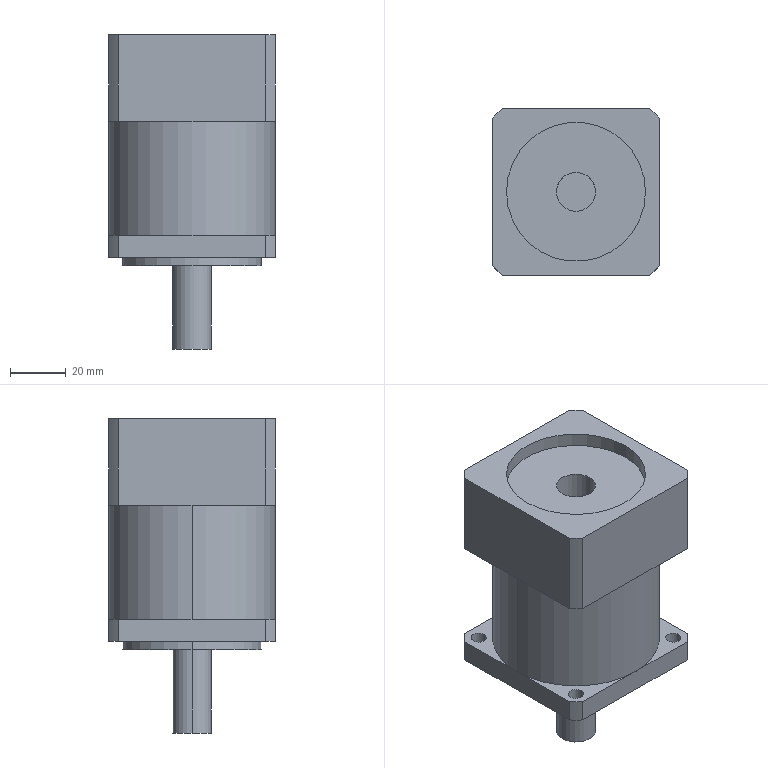Part | SolidWorks | features ICE 7, Extrusion 1, RefAxis 1, RevCut 1 | 1 solid | 48 faces | box 60 x 60 x 113 mm | volume 251469 mm3 | cylinder 26 | plane 22 | commonest cylinder face diameters 5.5 x8 80 x8 14 x4 50 x4 60 x2
STEP:
#1=CARTESIAN_POINT('',(-7.,0.,83.));
#2=VERTEX_POINT('',#1);
#3=CARTESIAN_POINT('',(7.,0.,83.));
#4=VERTEX_POINT('',#3);
#5=CARTESIAN_POINT('',(0.,0.,83.));
#6=DIRECTION('',(0.,0.,1.));
#7=DIRECTION('',(1.,0.,0.));
#8=AXIS2_PLACEMENT_3D('',#5,#6,#7);
#9=CIRCLE('',#8,7.);
#10=EDGE_CURVE('',#2,#4,#9,.T.);
#11=ORIENTED_EDGE('',*,*,#10,.F.);
#12=CARTESIAN_POINT('',(-7.,0.,108.));
#13=VERTEX_POINT('',#12);
#14=CARTESIAN_POINT('',(-7.,0.,83.));
#15=DIRECTION('',(0.,0.,1.));
#16=VECTOR('',#15,1000.);
#17=LINE('',#14,#16);
#18=EDGE_CURVE('',#2,#13,#17,.T.);
#19=ORIENTED_EDGE('',*,*,#18,.T.);
#20=CARTESIAN_POINT('',(7.,0.,108.));
#21=VERTEX_POINT('',#20);
#22=CARTESIAN_POINT('',(0.,0.,108.));
#23=DIRECTION('',(0.,0.,1.));
#24=DIRECTION('',(1.,0.,0.));
#25=AXIS2_PLACEMENT_3D('',#22,#23,#24);
#26=CIRCLE('',#25,7.);
#27=EDGE_CURVE('',#13,#21,#26,.T.);
#28=ORIENTED_EDGE('',*,*,#27,.T.);
#29=CARTESIAN_POINT('',(7.,0.,83.));
#30=DIRECTION('',(0.,0.,1.));
#31=VECTOR('',#30,1000.);
#32=LINE('',#29,#31);
#33=EDGE_CURVE('',#4,#21,#32,.T.);
#34=ORIENTED_EDGE('',*,*,#33,.F.);
#35=EDGE_LOOP('',(#11,#19,#28,#34));
#36=FACE_OUTER_BOUND('',#35,.T.);
#37=CARTESIAN_POINT('',(0.,0.,83.));
#38=DIRECTION('',(0.,0.,1.));
#39=DIRECTION('',(1.,0.,0.));
#40=AXIS2_PLACEMENT_3D('',#37,#38,#39);
#41=CYLINDRICAL_SURFACE('',#40,7.);
#42=ADVANCED_FACE('',(#36),#41,.F.);
#43=CARTESIAN_POINT('',(-25.,0.,108.));
#44=VERTEX_POINT('',#43);
#45=CARTESIAN_POINT('',(25.,0.,108.));
#46=VERTEX_POINT('',#45);
#47=CARTESIAN_POINT('',(0.,0.,108.));
#48=DIRECTION('',(0.,0.,1.));
#49=DIRECTION('',(1.,0.,0.));
#50=AXIS2_PLACEMENT_3D('',#47,#48,#49);
#51=CIRCLE('',#50,25.);
#52=EDGE_CURVE('',#44,#46,#51,.T.);
#53=ORIENTED_EDGE('',*,*,#52,.F.);
#54=CARTESIAN_POINT('',(-25.,0.,113.));
#55=VERTEX_POINT('',#54);
#56=CARTESIAN_POINT('',(-25.,0.,108.));
#57=DIRECTION('',(0.,0.,1.));
#58=VECTOR('',#57,1000.);
#59=LINE('',#56,#58);
#60=EDGE_CURVE('',#44,#55,#59,.T.);
#61=ORIENTED_EDGE('',*,*,#60,.T.);
#62=CARTESIAN_POINT('',(25.,0.,113.));
#63=VERTEX_POINT('',#62);
#64=CARTESIAN_POINT('',(0.,0.,113.));
#65=DIRECTION('',(0.,0.,1.));
#66=DIRECTION('',(1.,0.,0.));
#67=AXIS2_PLACEMENT_3D('',#64,#65,#66);
#68=CIRCLE('',#67,25.);
#69=EDGE_CURVE('',#55,#63,#68,.T.);
#70=ORIENTED_EDGE('',*,*,#69,.T.);
#71=CARTESIAN_POINT('',(25.,0.,108.));
#72=DIRECTION('',(0.,0.,1.));
#73=VECTOR('',#72,1000.);
#74=LINE('',#71,#73);
#75=EDGE_CURVE('',#46,#63,#74,.T.);
#76=ORIENTED_EDGE('',*,*,#75,.F.);
#77=EDGE_LOOP('',(#53,#61,#70,#76));
#78=FACE_OUTER_BOUND('',#77,.T.);
#79=CARTESIAN_POINT('',(0.,0.,108.));
#80=DIRECTION('',(0.,0.,1.));
#81=DIRECTION('',(1.,0.,0.));
#82=AXIS2_PLACEMENT_3D('',#79,#80,#81);
#83=CYLINDRICAL_SURFACE('',#82,25.);
#84=ADVANCED_FACE('',(#78),#83,.F.);
#85=CARTESIAN_POINT('',(-21.999,24.749,41.));
#86=VERTEX_POINT('',#85);
#87=CARTESIAN_POINT('',(-27.499,24.749,41.));
#88=VERTEX_POINT('',#87);
#89=CARTESIAN_POINT('',(-24.749,24.749,41.));
#90=DIRECTION('',(0.,0.,-1.));
#91=DIRECTION('',(1.,0.,0.));
#92=AXIS2_PLACEMENT_3D('',#89,#90,#91);
#93=CIRCLE('',#92,2.75);
#94=EDGE_CURVE('',#86,#88,#93,.T.);
#95=ORIENTED_EDGE('',*,*,#94,.F.);
#96=CARTESIAN_POINT('',(-21.999,24.749,33.));
#97=VERTEX_POINT('',#96);
#98=CARTESIAN_POINT('',(-21.999,24.749,113.001));
#99=DIRECTION('',(0.,0.,-1.));
#100=VECTOR('',#99,1000.);
#101=LINE('',#98,#100);
#102=EDGE_CURVE('',#86,#97,#101,.T.);
#103=ORIENTED_EDGE('',*,*,#102,.T.);
#104=CARTESIAN_POINT('',(-27.499,24.749,33.));
#105=VERTEX_POINT('',#104);
#106=CARTESIAN_POINT('',(-24.749,24.749,33.));
#107=DIRECTION('',(0.,0.,-1.));
#108=DIRECTION('',(1.,0.,0.));
#109=AXIS2_PLACEMENT_3D('',#106,#107,#108);
#110=CIRCLE('',#109,2.75);
#111=EDGE_CURVE('',#97,#105,#110,.T.);
#112=ORIENTED_EDGE('',*,*,#111,.T.);
#113=CARTESIAN_POINT('',(-27.499,24.749,113.001));
#114=DIRECTION('',(0.,0.,-1.));
#115=VECTOR('',#114,1000.);
#116=LINE('',#113,#115);
#117=EDGE_CURVE('',#88,#105,#116,.T.);
#118=ORIENTED_EDGE('',*,*,#117,.F.);
#119=EDGE_LOOP('',(#95,#103,#112,#118));
#120=FACE_OUTER_BOUND('',#119,.T.);
#121=CARTESIAN_POINT('',(-24.749,24.749,113.001));
#122=DIRECTION('',(0.,0.,-1.));
#123=DIRECTION('',(-1.,0.,0.));
#124=AXIS2_PLACEMENT_3D('',#121,#122,#123);
#125=CYLINDRICAL_SURFACE('',#124,2.75);
#126=ADVANCED_FACE('',(#120),#125,.F.);
#127=CARTESIAN_POINT('',(27.499,-24.749,41.));
#128=VERTEX_POINT('',#127);
#129=CARTESIAN_POINT('',(21.999,-24.749,41.));
#130=VERTEX_POINT('',#129);
#131=CARTESIAN_POINT('',(24.749,-24.749,41.));
#132=DIRECTION('',(0.,0.,-1.));
#133=DIRECTION('',(1.,0.,0.));
#134=AXIS2_PLACEMENT_3D('',#131,#132,#133);
#135=CIRCLE('',#134,2.75);
#136=EDGE_CURVE('',#128,#130,#135,.T.);
#137=ORIENTED_EDGE('',*,*,#136,.F.);
#138=CARTESIAN_POINT('',(27.499,-24.749,33.));
#139=VERTEX_POINT('',#138);
#140=CARTESIAN_POINT('',(27.499,-24.749,113.001));
#141=DIRECTION('',(0.,0.,-1.));
#142=VECTOR('',#141,1000.);
#143=LINE('',#140,#142);
#144=EDGE_CURVE('',#128,#139,#143,.T.);
#145=ORIENTED_EDGE('',*,*,#144,.T.);
#146=CARTESIAN_POINT('',(21.999,-24.749,33.));
#147=VERTEX_POINT('',#146);
#148=CARTESIAN_POINT('',(24.749,-24.749,33.));
#149=DIRECTION('',(0.,0.,-1.));
#150=DIRECTION('',(1.,0.,0.));
#151=AXIS2_PLACEMENT_3D('',#148,#149,#150);
#152=CIRCLE('',#151,2.75);
#153=EDGE_CURVE('',#139,#147,#152,.T.);
#154=ORIENTED_EDGE('',*,*,#153,.T.);
#155=CARTESIAN_POINT('',(21.999,-24.749,113.001));
#156=DIRECTION('',(0.,0.,-1.));
#157=VECTOR('',#156,1000.);
#158=LINE('',#155,#157);
#159=EDGE_CURVE('',#130,#147,#158,.T.);
#160=ORIENTED_EDGE('',*,*,#159,.F.);
#161=EDGE_LOOP('',(#137,#145,#154,#160));
#162=FACE_OUTER_BOUND('',#161,.T.);
#163=CARTESIAN_POINT('',(24.749,-24.749,113.001));
#164=DIRECTION('',(0.,0.,-1.));
#165=DIRECTION('',(-1.,0.,0.));
#166=AXIS2_PLACEMENT_3D('',#163,#164,#165);
#167=CYLINDRICAL_SURFACE('',#166,2.75);
#168=ADVANCED_FACE('',(#162),#167,.F.);
#169=CARTESIAN_POINT('',(-21.999,-24.749,41.));
#170=VERTEX_POINT('',#169);
#171=CARTESIAN_POINT('',(-27.499,-24.749,41.));
#172=VERTEX_POINT('',#171);
#173=CARTESIAN_POINT('',(-24.749,-24.749,41.));
#174=DIRECTION('',(0.,0.,-1.));
#175=DIRECTION('',(1.,0.,0.));
#176=AXIS2_PLACEMENT_3D('',#173,#174,#175);
#177=CIRCLE('',#176,2.75);
#178=EDGE_CURVE('',#170,#172,#177,.T.);
#179=ORIENTED_EDGE('',*,*,#178,.F.);
#180=CARTESIAN_POINT('',(-21.999,-24.749,33.));
#181=VERTEX_POINT('',#180);
#182=CARTESIAN_POINT('',(-21.999,-24.749,113.001));
#183=DIRECTION('',(0.,0.,-1.));
#184=VECTOR('',#183,1000.);
#185=LINE('',#182,#184);
#186=EDGE_CURVE('',#170,#181,#185,.T.);
#187=ORIENTED_EDGE('',*,*,#186,.T.);
#188=CARTESIAN_POINT('',(-27.499,-24.749,33.));
#189=VERTEX_POINT('',#188);
#190=CARTESIAN_POINT('',(-24.749,-24.749,33.));
#191=DIRECTION('',(0.,0.,-1.));
#192=DIRECTION('',(-1.,0.,0.));
#193=AXIS2_PLACEMENT_3D('',#190,#191,#192);
#194=CIRCLE('',#193,2.75);
#195=EDGE_CURVE('',#181,#189,#194,.T.);
#196=ORIENTED_EDGE('',*,*,#195,.T.);
#197=CARTESIAN_POINT('',(-27.499,-24.749,113.001));
#198=DIRECTION('',(0.,0.,-1.));
#199=VECTOR('',#198,1000.);
#200=LINE('',#197,#199);
#201=EDGE_CURVE('',#172,#189,#200,.T.);
#202=ORIENTED_EDGE('',*,*,#201,.F.);
#203=EDGE_LOOP('',(#179,#187,#196,#202));
#204=FACE_OUTER_BOUND('',#203,.T.);
#205=CARTESIAN_POINT('',(-24.749,-24.749,113.001));
#206=DIRECTION('',(0.,0.,-1.));
#207=DIRECTION('',(-1.,0.,0.));
#208=AXIS2_PLACEMENT_3D('',#205,#206,#207);
#209=CYLINDRICAL_SURFACE('',#208,2.75);
#210=ADVANCED_FACE('',(#204),#209,.F.);
#211=CARTESIAN_POINT('',(27.499,24.749,41.));
#212=VERTEX_POINT('',#211);
#213=CARTESIAN_POINT('',(21.999,24.749,41.));
#214=VERTEX_POINT('',#213);
#215=CARTESIAN_POINT('',(24.749,24.749,41.));
#216=DIRECTION('',(0.,0.,-1.));
#217=DIRECTION('',(1.,0.,0.));
#218=AXIS2_PLACEMENT_3D('',#215,#216,#217);
#219=CIRCLE('',#218,2.75);
#220=EDGE_CURVE('',#212,#214,#219,.T.);
#221=ORIENTED_EDGE('',*,*,#220,.F.);
#222=CARTESIAN_POINT('',(27.499,24.749,33.));
#223=VERTEX_POINT('',#222);
#224=CARTESIAN_POINT('',(27.499,24.749,113.001));
#225=DIRECTION('',(0.,0.,-1.));
#226=VECTOR('',#225,1000.);
#227=LINE('',#224,#226);
#228=EDGE_CURVE('',#212,#223,#227,.T.);
#229=ORIENTED_EDGE('',*,*,#228,.T.);
#230=CARTESIAN_POINT('',(21.999,24.749,33.));
#231=VERTEX_POINT('',#230);
#232=CARTESIAN_POINT('',(24.749,24.749,33.));
#233=DIRECTION('',(0.,0.,-1.));
#234=DIRECTION('',(-1.,0.,0.));
#235=AXIS2_PLACEMENT_3D('',#232,#233,#234);
#236=CIRCLE('',#235,2.75);
#237=EDGE_CURVE('',#223,#231,#236,.T.);
#238=ORIENTED_EDGE('',*,*,#237,.T.);
#239=CARTESIAN_POINT('',(21.999,24.749,113.001));
#240=DIRECTION('',(0.,0.,-1.));
#241=VECTOR('',#240,1000.);
#242=LINE('',#239,#241);
#243=EDGE_CURVE('',#214,#231,#242,.T.);
#244=ORIENTED_EDGE('',*,*,#243,.F.);
#245=EDGE_LOOP('',(#221,#229,#238,#244));
#246=FACE_OUTER_BOUND('',#245,.T.);
#247=CARTESIAN_POINT('',(24.749,24.749,113.001));
#248=DIRECTION('',(0.,0.,-1.));
#249=DIRECTION('',(-1.,0.,0.));
#250=AXIS2_PLACEMENT_3D('',#247,#248,#249);
#251=CYLINDRICAL_SURFACE('',#250,2.75);
#252=ADVANCED_FACE('',(#246),#251,.F.);
#253=CARTESIAN_POINT('',(30.,0.,82.));
#254=VERTEX_POINT('',#253);
#255=CARTESIAN_POINT('',(0.,30.,82.));
#256=VERTEX_POINT('',#255);
#257=CARTESIAN_POINT('',(0.,0.,82.));
#258=DIRECTION('',(0.,0.,1.));
#259=DIRECTION('',(1.,0.,0.));
#260=AXIS2_PLACEMENT_3D('',#257,#258,#259);
#261=CIRCLE('',#260,30.);
#262=EDGE_CURVE('',#254,#256,#261,.T.);
#263=ORIENTED_EDGE('',*,*,#262,.F.);
#264=CARTESIAN_POINT('',(30.,0.,41.));
#265=VERTEX_POINT('',#264);
#266=CARTESIAN_POINT('',(30.,0.,82.));
#267=DIRECTION('',(0.,0.,-1.));
#268=VECTOR('',#267,1000.);
#269=LINE('',#266,#268);
#270=EDGE_CURVE('',#254,#265,#269,.T.);
#271=ORIENTED_EDGE('',*,*,#270,.T.);
#272=CARTESIAN_POINT('',(0.,30.,41.));
#273=VERTEX_POINT('',#272);
#274=CARTESIAN_POINT('',(0.,0.,41.));
#275=DIRECTION('',(0.,0.,1.));
#276=DIRECTION('',(1.,0.,0.));
#277=AXIS2_PLACEMENT_3D('',#274,#275,#276);
#278=CIRCLE('',#277,30.);
#279=EDGE_CURVE('',#265,#273,#278,.T.);
#280=ORIENTED_EDGE('',*,*,#279,.T.);
#281=CARTESIAN_POINT('',(-30.,0.,41.));
#282=VERTEX_POINT('',#281);
#283=CARTESIAN_POINT('',(0.,0.,41.));
#284=DIRECTION('',(0.,0.,1.));
#285=DIRECTION('',(1.,0.,0.));
#286=AXIS2_PLACEMENT_3D('',#283,#284,#285);
#287=CIRCLE('',#286,30.);
#288=EDGE_CURVE('',#273,#282,#287,.T.);
#289=ORIENTED_EDGE('',*,*,#288,.T.);
#290=CARTESIAN_POINT('',(-30.,0.,82.));
#291=VERTEX_POINT('',#290);
#292=CARTESIAN_POINT('',(-30.,0.,82.));
#293=DIRECTION('',(0.,0.,-1.));
#294=VECTOR('',#293,1000.);
#295=LINE('',#292,#294);
#296=EDGE_CURVE('',#291,#282,#295,.T.);
#297=ORIENTED_EDGE('',*,*,#296,.F.);
#298=CARTESIAN_POINT('',(0.,0.,82.));
#299=DIRECTION('',(0.,0.,1.));
#300=DIRECTION('',(1.,0.,0.));
#301=AXIS2_PLACEMENT_3D('',#298,#299,#300);
#302=CIRCLE('',#301,30.);
#303=EDGE_CURVE('',#256,#291,#302,.T.);
#304=ORIENTED_EDGE('',*,*,#303,.F.);
#305=EDGE_LOOP('',(#263,#271,#280,#289,#297,#304));
#306=FACE_OUTER_BOUND('',#305,.T.);
#307=CARTESIAN_POINT('',(0.,0.,82.));
#308=DIRECTION('',(0.,0.,-1.));
#309=DIRECTION('',(-1.,0.,0.));
#310=AXIS2_PLACEMENT_3D('',#307,#308,#309);
#311=CYLINDRICAL_SURFACE('',#310,30.);
#312=ADVANCED_FACE('',(#306),#311,.T.);
#313=CARTESIAN_POINT('',(25.,0.,33.));
#314=VERTEX_POINT('',#313);
#315=CARTESIAN_POINT('',(-25.,0.,33.));
#316=VERTEX_POINT('',#315);
#317=CARTESIAN_POINT('',(0.,0.,33.));
#318=DIRECTION('',(0.,0.,1.));
#319=DIRECTION('',(1.,0.,0.));
#320=AXIS2_PLACEMENT_3D('',#317,#318,#319);
#321=CIRCLE('',#320,25.);
#322=EDGE_CURVE('',#314,#316,#321,.T.);
#323=ORIENTED_EDGE('',*,*,#322,.F.);
#324=CARTESIAN_POINT('',(25.,0.,30.));
#325=VERTEX_POINT('',#324);
#326=CARTESIAN_POINT('',(25.,0.,33.));
#327=DIRECTION('',(0.,0.,-1.));
#328=VECTOR('',#327,1000.);
#329=LINE('',#326,#328);
#330=EDGE_CURVE('',#314,#325,#329,.T.);
#331=ORIENTED_EDGE('',*,*,#330,.T.);
#332=CARTESIAN_POINT('',(-25.,0.,30.));
#333=VERTEX_POINT('',#332);
#334=CARTESIAN_POINT('',(0.,0.,30.));
#335=DIRECTION('',(0.,0.,1.));
#336=DIRECTION('',(1.,0.,0.));
#337=AXIS2_PLACEMENT_3D('',#334,#335,#336);
#338=CIRCLE('',#337,25.);
#339=EDGE_CURVE('',#325,#333,#338,.T.);
#340=ORIENTED_EDGE('',*,*,#339,.T.);
#341=CARTESIAN_POINT('',(-25.,0.,33.));
#342=DIRECTION('',(0.,0.,-1.));
#343=VECTOR('',#342,1000.);
#344=LINE('',#341,#343);
#345=EDGE_CURVE('',#316,#333,#344,.T.);
#346=ORIENTED_EDGE('',*,*,#345,.F.);
#347=EDGE_LOOP('',(#323,#331,#340,#346));
#348=FACE_OUTER_BOUND('',#347,.T.);
#349=CARTESIAN_POINT('',(0.,0.,33.));
#350=DIRECTION('',(0.,0.,-1.));
#351=DIRECTION('',(-1.,0.,0.));
#352=AXIS2_PLACEMENT_3D('',#349,#350,#351);
#353=CYLINDRICAL_SURFACE('',#352,25.);
#354=ADVANCED_FACE('',(#348),#353,.T.);
#355=CARTESIAN_POINT('',(7.,0.,30.));
#356=VERTEX_POINT('',#355);
#357=CARTESIAN_POINT('',(-7.,0.,30.));
#358=VERTEX_POINT('',#357);
#359=CARTESIAN_POINT('',(0.,0.,30.));
#360=DIRECTION('',(0.,0.,1.));
#361=DIRECTION('',(1.,0.,0.));
#362=AXIS2_PLACEMENT_3D('',#359,#360,#361);
#363=CIRCLE('',#362,7.);
#364=EDGE_CURVE('',#356,#358,#363,.T.);
#365=ORIENTED_EDGE('',*,*,#364,.F.);
#366=CARTESIAN_POINT('',(7.,0.,0.));
#367=VERTEX_POINT('',#366);
#368=CARTESIAN_POINT('',(7.,0.,30.));
#369=DIRECTION('',(0.,0.,-1.));
#370=VECTOR('',#369,1000.);
#371=LINE('',#368,#370);
#372=EDGE_CURVE('',#356,#367,#371,.T.);
#373=ORIENTED_EDGE('',*,*,#372,.T.);
#374=CARTESIAN_POINT('',(-7.,0.,0.));
#375=VERTEX_POINT('',#374);
#376=CARTESIAN_POINT('',(0.,0.,0.));
#377=DIRECTION('',(0.,0.,1.));
#378=DIRECTION('',(1.,0.,0.));
#379=AXIS2_PLACEMENT_3D('',#376,#377,#378);
#380=CIRCLE('',#379,7.);
#381=EDGE_CURVE('',#367,#375,#380,.T.);
#382=ORIENTED_EDGE('',*,*,#381,.T.);
#383=CARTESIAN_POINT('',(-7.,0.,30.));
#384=DIRECTION('',(0.,0.,-1.));
#385=VECTOR('',#384,1000.);
#386=LINE('',#383,#385);
#387=EDGE_CURVE('',#358,#375,#386,.T.);
#388=ORIENTED_EDGE('',*,*,#387,.F.);
#389=EDGE_LOOP('',(#365,#373,#382,#388));
#390=FACE_OUTER_BOUND('',#389,.T.);
#391=CARTESIAN_POINT('',(0.,0.,30.));
#392=DIRECTION('',(0.,0.,-1.));
#393=DIRECTION('',(-1.,0.,0.));
#394=AXIS2_PLACEMENT_3D('',#391,#392,#393);
#395=CYLINDRICAL_SURFACE('',#394,7.);
#396=ADVANCED_FACE('',(#390),#395,.T.);
#397=CARTESIAN_POINT('',(24.749,24.749,41.));
#398=DIRECTION('',(0.,0.,-1.));
#399=DIRECTION('',(1.,0.,0.));
#400=AXIS2_PLACEMENT_3D('',#397,#398,#399);
#401=CIRCLE('',#400,2.75);
#402=EDGE_CURVE('',#214,#212,#401,.T.);
#403=ORIENTED_EDGE('',*,*,#402,.T.);
#404=ORIENTED_EDGE('',*,*,#220,.T.);
#405=EDGE_LOOP('',(#403,#404));
#406=FACE_BOUND('',#405,.T.);
#407=CARTESIAN_POINT('',(30.,26.458,41.));
#408=VERTEX_POINT('',#407);
#409=CARTESIAN_POINT('',(30.,30.,41.));
#410=DIRECTION('',(0.,1.,0.));
#411=VECTOR('',#410,1000.);
#412=LINE('',#409,#411);
#413=EDGE_CURVE('',#265,#408,#412,.T.);
#414=ORIENTED_EDGE('',*,*,#413,.T.);
#415=CARTESIAN_POINT('',(26.458,30.,41.));
#416=VERTEX_POINT('',#415);
#417=CARTESIAN_POINT('',(0.,0.,41.));
#418=DIRECTION('',(0.,0.,1.));
#419=DIRECTION('',(1.,0.,0.));
#420=AXIS2_PLACEMENT_3D('',#417,#418,#419);
#421=CIRCLE('',#420,40.);
#422=EDGE_CURVE('',#408,#416,#421,.T.);
#423=ORIENTED_EDGE('',*,*,#422,.T.);
#424=CARTESIAN_POINT('',(-30.,30.,41.));
#425=DIRECTION('',(-1.,0.,0.));
#426=VECTOR('',#425,1000.);
#427=LINE('',#424,#426);
#428=EDGE_CURVE('',#416,#273,#427,.T.);
#429=ORIENTED_EDGE('',*,*,#428,.T.);
#430=ORIENTED_EDGE('',*,*,#279,.F.);
#431=EDGE_LOOP('',(#414,#423,#429,#430));
#432=FACE_OUTER_BOUND('',#431,.T.);
#433=CARTESIAN_POINT('',(0.,0.,41.));
#434=DIRECTION('',(0.,0.,1.));
#435=DIRECTION('',(1.,0.,0.));
#436=AXIS2_PLACEMENT_3D('',#433,#434,#435);
#437=PLANE('',#436);
#438=ADVANCED_FACE('',(#406,#432),#437,.T.);
#439=CARTESIAN_POINT('',(-24.749,24.749,41.));
#440=DIRECTION('',(0.,0.,-1.));
#441=DIRECTION('',(1.,0.,0.));
#442=AXIS2_PLACEMENT_3D('',#439,#440,#441);
#443=CIRCLE('',#442,2.75);
#444=EDGE_CURVE('',#88,#86,#443,.T.);
#445=ORIENTED_EDGE('',*,*,#444,.T.);
#446=ORIENTED_EDGE('',*,*,#94,.T.);
#447=EDGE_LOOP('',(#445,#446));
#448=FACE_BOUND('',#447,.T.);
#449=CARTESIAN_POINT('',(-26.458,30.,41.));
#450=VERTEX_POINT('',#449);
#451=CARTESIAN_POINT('',(-30.,30.,41.));
#452=DIRECTION('',(-1.,0.,0.));
#453=VECTOR('',#452,1000.);
#454=LINE('',#451,#453);
#455=EDGE_CURVE('',#273,#450,#454,.T.);
#456=ORIENTED_EDGE('',*,*,#455,.T.);
#457=CARTESIAN_POINT('',(-30.,26.458,41.));
#458=VERTEX_POINT('',#457);
#459=CARTESIAN_POINT('',(0.,0.,41.));
#460=DIRECTION('',(0.,0.,1.));
#461=DIRECTION('',(1.,0.,0.));
#462=AXIS2_PLACEMENT_3D('',#459,#460,#461);
#463=CIRCLE('',#462,40.);
#464=EDGE_CURVE('',#450,#458,#463,.T.);
#465=ORIENTED_EDGE('',*,*,#464,.T.);
#466=CARTESIAN_POINT('',(-30.,30.,41.));
#467=DIRECTION('',(0.,-1.,0.));
#468=VECTOR('',#467,1000.);
#469=LINE('',#466,#468);
#470=EDGE_CURVE('',#458,#282,#469,.T.);
#471=ORIENTED_EDGE('',*,*,#470,.T.);
#472=ORIENTED_EDGE('',*,*,#288,.F.);
#473=EDGE_LOOP('',(#456,#465,#471,#472));
#474=FACE_OUTER_BOUND('',#473,.T.);
#475=CARTESIAN_POINT('',(0.,0.,41.));
#476=DIRECTION('',(0.,0.,1.));
#477=DIRECTION('',(1.,0.,0.));
#478=AXIS2_PLACEMENT_3D('',#475,#476,#477);
#479=PLANE('',#478);
#480=ADVANCED_FACE('',(#448,#474),#479,.T.);
#481=CARTESIAN_POINT('',(-24.749,-24.749,41.));
#482=DIRECTION('',(0.,0.,-1.));
#483=DIRECTION('',(1.,0.,0.));
#484=AXIS2_PLACEMENT_3D('',#481,#482,#483);
#485=CIRCLE('',#484,2.75);
#486=EDGE_CURVE('',#172,#170,#485,.T.);
#487=ORIENTED_EDGE('',*,*,#486,.T.);
#488=ORIENTED_EDGE('',*,*,#178,.T.);
#489=EDGE_LOOP('',(#487,#488));
#490=FACE_BOUND('',#489,.T.);
#491=CARTESIAN_POINT('',(-30.,-26.458,41.));
#492=VERTEX_POINT('',#491);
#493=CARTESIAN_POINT('',(-30.,30.,41.));
#494=DIRECTION('',(0.,-1.,0.));
#495=VECTOR('',#494,1000.);
#496=LINE('',#493,#495);
#497=EDGE_CURVE('',#282,#492,#496,.T.);
#498=ORIENTED_EDGE('',*,*,#497,.T.);
#499=CARTESIAN_POINT('',(-26.458,-30.,41.));
#500=VERTEX_POINT('',#499);
#501=CARTESIAN_POINT('',(0.,0.,41.));
#502=DIRECTION('',(0.,0.,1.));
#503=DIRECTION('',(1.,0.,0.));
#504=AXIS2_PLACEMENT_3D('',#501,#502,#503);
#505=CIRCLE('',#504,40.);
#506=EDGE_CURVE('',#492,#500,#505,.T.);
#507=ORIENTED_EDGE('',*,*,#506,.T.);
#508=CARTESIAN_POINT('',(0.,-30.,41.));
#509=VERTEX_POINT('',#508);
#510=CARTESIAN_POINT('',(-30.,-30.,41.));
#511=DIRECTION('',(1.,0.,0.));
#512=VECTOR('',#511,1000.);
#513=LINE('',#510,#512);
#514=EDGE_CURVE('',#500,#509,#513,.T.);
#515=ORIENTED_EDGE('',*,*,#514,.T.);
#516=CARTESIAN_POINT('',(0.,0.,41.));
#517=DIRECTION('',(0.,0.,1.));
#518=DIRECTION('',(1.,0.,0.));
#519=AXIS2_PLACEMENT_3D('',#516,#517,#518);
#520=CIRCLE('',#519,30.);
#521=EDGE_CURVE('',#282,#509,#520,.T.);
#522=ORIENTED_EDGE('',*,*,#521,.F.);
#523=EDGE_LOOP('',(#498,#507,#515,#522));
#524=FACE_OUTER_BOUND('',#523,.T.);
#525=CARTESIAN_POINT('',(0.,0.,41.));
#526=DIRECTION('',(0.,0.,1.));
#527=DIRECTION('',(1.,0.,0.));
#528=AXIS2_PLACEMENT_3D('',#525,#526,#527);
#529=PLANE('',#528);
#530=ADVANCED_FACE('',(#490,#524),#529,.T.);
#531=CARTESIAN_POINT('',(30.,-26.458,33.));
#532=VERTEX_POINT('',#531);
#533=CARTESIAN_POINT('',(30.,-26.458,41.));
#534=VERTEX_POINT('',#533);
#535=CARTESIAN_POINT('',(30.,-26.458,82.));
#536=DIRECTION('',(0.,0.,1.));
#537=VECTOR('',#536,1000.);
#538=LINE('',#535,#537);
#539=EDGE_CURVE('',#532,#534,#538,.T.);
#540=ORIENTED_EDGE('',*,*,#539,.F.);
#541=CARTESIAN_POINT('',(30.,26.458,33.));
#542=VERTEX_POINT('',#541);
#543=CARTESIAN_POINT('',(30.,30.,33.));
#544=DIRECTION('',(0.,1.,0.));
#545=VECTOR('',#544,1000.);
#546=LINE('',#543,#545);
#547=EDGE_CURVE('',#532,#542,#546,.T.);
#548=ORIENTED_EDGE('',*,*,#547,.T.);
#549=CARTESIAN_POINT('',(30.,26.458,82.));
#550=DIRECTION('',(0.,0.,-1.));
#551=VECTOR('',#550,1000.);
#552=LINE('',#549,#551);
#553=EDGE_CURVE('',#408,#542,#552,.T.);
#554=ORIENTED_EDGE('',*,*,#553,.F.);
#555=ORIENTED_EDGE('',*,*,#413,.F.);
#556=CARTESIAN_POINT('',(30.,30.,41.));
#557=DIRECTION('',(0.,1.,0.));
#558=VECTOR('',#557,1000.);
#559=LINE('',#556,#558);
#560=EDGE_CURVE('',#534,#265,#559,.T.);
#561=ORIENTED_EDGE('',*,*,#560,.F.);
#562=EDGE_LOOP('',(#540,#548,#554,#555,#561));
#563=FACE_OUTER_BOUND('',#562,.T.);
#564=CARTESIAN_POINT('',(30.,30.,41.));
#565=DIRECTION('',(-1.,0.,0.));
#566=DIRECTION('',(0.,-1.,0.));
#567=AXIS2_PLACEMENT_3D('',#564,#565,#566);
#568=PLANE('',#567);
#569=ADVANCED_FACE('',(#563),#568,.F.);
#570=CARTESIAN_POINT('',(26.458,30.,33.));
#571=VERTEX_POINT('',#570);
#572=CARTESIAN_POINT('',(26.458,30.,82.));
#573=DIRECTION('',(0.,0.,1.));
#574=VECTOR('',#573,1000.);
#575=LINE('',#572,#574);
#576=EDGE_CURVE('',#571,#416,#575,.T.);
#577=ORIENTED_EDGE('',*,*,#576,.F.);
#578=CARTESIAN_POINT('',(-26.458,30.,33.));
#579=VERTEX_POINT('',#578);
#580=CARTESIAN_POINT('',(-30.,30.,33.));
#581=DIRECTION('',(-1.,0.,0.));
#582=VECTOR('',#581,1000.);
#583=LINE('',#580,#582);
#584=EDGE_CURVE('',#571,#579,#583,.T.);
#585=ORIENTED_EDGE('',*,*,#584,.T.);
#586=CARTESIAN_POINT('',(-26.458,30.,82.));
#587=DIRECTION('',(0.,0.,-1.));
#588=VECTOR('',#587,1000.);
#589=LINE('',#586,#588);
#590=EDGE_CURVE('',#450,#579,#589,.T.);
#591=ORIENTED_EDGE('',*,*,#590,.F.);
#592=ORIENTED_EDGE('',*,*,#455,.F.);
#593=ORIENTED_EDGE('',*,*,#428,.F.);
#594=EDGE_LOOP('',(#577,#585,#591,#592,#593));
#595=FACE_OUTER_BOUND('',#594,.T.);
#596=CARTESIAN_POINT('',(-30.,30.,41.));
#597=DIRECTION('',(0.,-1.,0.));
#598=DIRECTION('',(0.,0.,-1.));
#599=AXIS2_PLACEMENT_3D('',#596,#597,#598);
#600=PLANE('',#599);
#601=ADVANCED_FACE('',(#595),#600,.F.);
#602=CARTESIAN_POINT('',(-30.,26.458,33.));
#603=VERTEX_POINT('',#602);
#604=CARTESIAN_POINT('',(-30.,26.458,82.));
#605=DIRECTION('',(0.,0.,1.));
#606=VECTOR('',#605,1000.);
#607=LINE('',#604,#606);
#608=EDGE_CURVE('',#603,#458,#607,.T.);
#609=ORIENTED_EDGE('',*,*,#608,.F.);
#610=CARTESIAN_POINT('',(-30.,-26.458,33.));
#611=VERTEX_POINT('',#610);
#612=CARTESIAN_POINT('',(-30.,30.,33.));
#613=DIRECTION('',(0.,-1.,0.));
#614=VECTOR('',#613,1000.);
#615=LINE('',#612,#614);
#616=EDGE_CURVE('',#603,#611,#615,.T.);
#617=ORIENTED_EDGE('',*,*,#616,.T.);
#618=CARTESIAN_POINT('',(-30.,-26.458,82.));
#619=DIRECTION('',(0.,0.,-1.));
#620=VECTOR('',#619,1000.);
#621=LINE('',#618,#620);
#622=EDGE_CURVE('',#492,#611,#621,.T.);
#623=ORIENTED_EDGE('',*,*,#622,.F.);
#624=ORIENTED_EDGE('',*,*,#497,.F.);
#625=ORIENTED_EDGE('',*,*,#470,.F.);
#626=EDGE_LOOP('',(#609,#617,#623,#624,#625));
#627=FACE_OUTER_BOUND('',#626,.T.);
#628=CARTESIAN_POINT('',(-30.,30.,41.));
#629=DIRECTION('',(1.,0.,0.));
#630=DIRECTION('',(0.,1.,0.));
#631=AXIS2_PLACEMENT_3D('',#628,#629,#630);
#632=PLANE('',#631);
#633=ADVANCED_FACE('',(#627),#632,.F.);
#634=CARTESIAN_POINT('',(-26.458,-30.,33.));
#635=VERTEX_POINT('',#634);
#636=CARTESIAN_POINT('',(-26.458,-30.,82.));
#637=DIRECTION('',(0.,0.,1.));
#638=VECTOR('',#637,1000.);
#639=LINE('',#636,#638);
#640=EDGE_CURVE('',#635,#500,#639,.T.);
#641=ORIENTED_EDGE('',*,*,#640,.F.);
#642=CARTESIAN_POINT('',(26.458,-30.,33.));
#643=VERTEX_POINT('',#642);
#644=CARTESIAN_POINT('',(-30.,-30.,33.));
#645=DIRECTION('',(1.,0.,0.));
#646=VECTOR('',#645,1000.);
#647=LINE('',#644,#646);
#648=EDGE_CURVE('',#635,#643,#647,.T.);
#649=ORIENTED_EDGE('',*,*,#648,.T.);
#650=CARTESIAN_POINT('',(26.458,-30.,41.));
#651=VERTEX_POINT('',#650);
#652=CARTESIAN_POINT('',(26.458,-30.,82.));
#653=DIRECTION('',(0.,0.,-1.));
#654=VECTOR('',#653,1000.);
#655=LINE('',#652,#654);
#656=EDGE_CURVE('',#651,#643,#655,.T.);
#657=ORIENTED_EDGE('',*,*,#656,.F.);
#658=CARTESIAN_POINT('',(-30.,-30.,41.));
#659=DIRECTION('',(1.,0.,0.));
#660=VECTOR('',#659,1000.);
#661=LINE('',#658,#660);
#662=EDGE_CURVE('',#509,#651,#661,.T.);
#663=ORIENTED_EDGE('',*,*,#662,.F.);
#664=ORIENTED_EDGE('',*,*,#514,.F.);
#665=EDGE_LOOP('',(#641,#649,#657,#663,#664));
#666=FACE_OUTER_BOUND('',#665,.T.);
#667=CARTESIAN_POINT('',(-30.,-30.,41.));
#668=DIRECTION('',(0.,1.,0.));
#669=DIRECTION('',(0.,0.,1.));
#670=AXIS2_PLACEMENT_3D('',#667,#668,#669);
#671=PLANE('',#670);
#672=ADVANCED_FACE('',(#666),#671,.F.);
#673=CARTESIAN_POINT('',(24.749,-24.749,41.));
#674=DIRECTION('',(0.,0.,-1.));
#675=DIRECTION('',(1.,0.,0.));
#676=AXIS2_PLACEMENT_3D('',#673,#674,#675);
#677=CIRCLE('',#676,2.75);
#678=EDGE_CURVE('',#130,#128,#677,.T.);
#679=ORIENTED_EDGE('',*,*,#678,.T.);
#680=ORIENTED_EDGE('',*,*,#136,.T.);
#681=EDGE_LOOP('',(#679,#680));
#682=FACE_BOUND('',#681,.T.);
#683=ORIENTED_EDGE('',*,*,#662,.T.);
#684=CARTESIAN_POINT('',(0.,0.,41.));
#685=DIRECTION('',(0.,0.,1.));
#686=DIRECTION('',(1.,0.,0.));
#687=AXIS2_PLACEMENT_3D('',#684,#685,#686);
#688=CIRCLE('',#687,40.);
#689=EDGE_CURVE('',#651,#534,#688,.T.);
#690=ORIENTED_EDGE('',*,*,#689,.T.);
#691=ORIENTED_EDGE('',*,*,#560,.T.);
#692=CARTESIAN_POINT('',(0.,0.,41.));
#693=DIRECTION('',(0.,0.,1.));
#694=DIRECTION('',(1.,0.,0.));
#695=AXIS2_PLACEMENT_3D('',#692,#693,#694);
#696=CIRCLE('',#695,30.);
#697=EDGE_CURVE('',#509,#265,#696,.T.);
#698=ORIENTED_EDGE('',*,*,#697,.F.);
#699=EDGE_LOOP('',(#683,#690,#691,#698));
#700=FACE_OUTER_BOUND('',#699,.T.);
#701=CARTESIAN_POINT('',(0.,0.,41.));
#702=DIRECTION('',(0.,0.,1.));
#703=DIRECTION('',(1.,0.,0.));
#704=AXIS2_PLACEMENT_3D('',#701,#702,#703);
#705=PLANE('',#704);
#706=ADVANCED_FACE('',(#682,#700),#705,.T.);
#707=CARTESIAN_POINT('',(-24.749,24.749,33.));
#708=DIRECTION('',(0.,0.,-1.));
#709=DIRECTION('',(1.,0.,0.));
#710=AXIS2_PLACEMENT_3D('',#707,#708,#709);
#711=CIRCLE('',#710,2.75);
#712=EDGE_CURVE('',#105,#97,#711,.T.);
#713=ORIENTED_EDGE('',*,*,#712,.F.);
#714=ORIENTED_EDGE('',*,*,#111,.F.);
#715=EDGE_LOOP('',(#713,#714));
#716=FACE_BOUND('',#715,.T.);
#717=CARTESIAN_POINT('',(24.749,-24.749,33.));
#718=DIRECTION('',(0.,0.,-1.));
#719=DIRECTION('',(1.,0.,0.));
#720=AXIS2_PLACEMENT_3D('',#717,#718,#719);
#721=CIRCLE('',#720,2.75);
#722=EDGE_CURVE('',#147,#139,#721,.T.);
#723=ORIENTED_EDGE('',*,*,#722,.F.);
#724=ORIENTED_EDGE('',*,*,#153,.F.);
#725=EDGE_LOOP('',(#723,#724));
#726=FACE_BOUND('',#725,.T.);
#727=CARTESIAN_POINT('',(-24.749,-24.749,33.));
#728=DIRECTION('',(0.,0.,-1.));
#729=DIRECTION('',(-1.,0.,0.));
#730=AXIS2_PLACEMENT_3D('',#727,#728,#729);
#731=CIRCLE('',#730,2.75);
#732=EDGE_CURVE('',#189,#181,#731,.T.);
#733=ORIENTED_EDGE('',*,*,#732,.F.);
#734=ORIENTED_EDGE('',*,*,#195,.F.);
#735=EDGE_LOOP('',(#733,#734));
#736=FACE_BOUND('',#735,.T.);
#737=CARTESIAN_POINT('',(24.749,24.749,33.));
#738=DIRECTION('',(0.,0.,-1.));
#739=DIRECTION('',(-1.,0.,0.));
#740=AXIS2_PLACEMENT_3D('',#737,#738,#739);
#741=CIRCLE('',#740,2.75);
#742=EDGE_CURVE('',#231,#223,#741,.T.);
#743=ORIENTED_EDGE('',*,*,#742,.F.);
#744=ORIENTED_EDGE('',*,*,#237,.F.);
#745=EDGE_LOOP('',(#743,#744));
#746=FACE_BOUND('',#745,.T.);
#747=CARTESIAN_POINT('',(0.,0.,33.));
#748=DIRECTION('',(0.,0.,1.));
#749=DIRECTION('',(1.,0.,0.));
#750=AXIS2_PLACEMENT_3D('',#747,#748,#749);
#751=CIRCLE('',#750,25.);
#752=EDGE_CURVE('',#316,#314,#751,.T.);
#753=ORIENTED_EDGE('',*,*,#752,.T.);
#754=ORIENTED_EDGE('',*,*,#322,.T.);
#755=EDGE_LOOP('',(#753,#754));
#756=FACE_BOUND('',#755,.T.);
#757=CARTESIAN_POINT('',(0.,0.,33.));
#758=DIRECTION('',(0.,0.,1.));
#759=DIRECTION('',(1.,0.,0.));
#760=AXIS2_PLACEMENT_3D('',#757,#758,#759);
#761=CIRCLE('',#760,40.);
#762=EDGE_CURVE('',#542,#571,#761,.T.);
#763=ORIENTED_EDGE('',*,*,#762,.F.);
#764=ORIENTED_EDGE('',*,*,#547,.F.);
#765=CARTESIAN_POINT('',(0.,0.,33.));
#766=DIRECTION('',(0.,0.,1.));
#767=DIRECTION('',(1.,0.,0.));
#768=AXIS2_PLACEMENT_3D('',#765,#766,#767);
#769=CIRCLE('',#768,40.);
#770=EDGE_CURVE('',#643,#532,#769,.T.);
#771=ORIENTED_EDGE('',*,*,#770,.F.);
#772=ORIENTED_EDGE('',*,*,#648,.F.);
#773=CARTESIAN_POINT('',(0.,0.,33.));
#774=DIRECTION('',(0.,0.,1.));
#775=DIRECTION('',(1.,0.,0.));
#776=AXIS2_PLACEMENT_3D('',#773,#774,#775);
#777=CIRCLE('',#776,40.);
#778=EDGE_CURVE('',#611,#635,#777,.T.);
#779=ORIENTED_EDGE('',*,*,#778,.F.);
#780=ORIENTED_EDGE('',*,*,#616,.F.);
#781=CARTESIAN_POINT('',(0.,0.,33.));
#782=DIRECTION('',(0.,0.,1.));
#783=DIRECTION('',(1.,0.,0.));
#784=AXIS2_PLACEMENT_3D('',#781,#782,#783);
#785=CIRCLE('',#784,40.);
#786=EDGE_CURVE('',#579,#603,#785,.T.);
#787=ORIENTED_EDGE('',*,*,#786,.F.);
#788=ORIENTED_EDGE('',*,*,#584,.F.);
#789=EDGE_LOOP('',(#763,#764,#771,#772,#779,#780,#787,#788));
#790=FACE_OUTER_BOUND('',#789,.T.);
#791=CARTESIAN_POINT('',(0.,0.,33.));
#792=DIRECTION('',(0.,0.,1.));
#793=DIRECTION('',(1.,0.,0.));
#794=AXIS2_PLACEMENT_3D('',#791,#792,#793);
#795=PLANE('',#794);
#796=ADVANCED_FACE('',(#716,#726,#736,#746,#756,#790),#795,.F.);
#797=CARTESIAN_POINT('',(30.,26.458,82.));
#798=VERTEX_POINT('',#797);
#799=CARTESIAN_POINT('',(26.458,30.,82.));
#800=VERTEX_POINT('',#799);
#801=CARTESIAN_POINT('',(0.,0.,82.));
#802=DIRECTION('',(0.,0.,1.));
#803=DIRECTION('',(1.,0.,0.));
#804=AXIS2_PLACEMENT_3D('',#801,#802,#803);
#805=CIRCLE('',#804,40.);
#806=EDGE_CURVE('',#798,#800,#805,.T.);
#807=ORIENTED_EDGE('',*,*,#806,.F.);
#808=CARTESIAN_POINT('',(30.,30.,82.));
#809=DIRECTION('',(0.,1.,0.));
#810=VECTOR('',#809,1000.);
#811=LINE('',#808,#810);
#812=EDGE_CURVE('',#254,#798,#811,.T.);
#813=ORIENTED_EDGE('',*,*,#812,.F.);
#814=ORIENTED_EDGE('',*,*,#262,.T.);
#815=CARTESIAN_POINT('',(-30.,30.,82.));
#816=DIRECTION('',(-1.,0.,0.));
#817=VECTOR('',#816,1000.);
#818=LINE('',#815,#817);
#819=EDGE_CURVE('',#800,#256,#818,.T.);
#820=ORIENTED_EDGE('',*,*,#819,.F.);
#821=EDGE_LOOP('',(#807,#813,#814,#820));
#822=FACE_OUTER_BOUND('',#821,.T.);
#823=CARTESIAN_POINT('',(0.,0.,82.));
#824=DIRECTION('',(0.,0.,1.));
#825=DIRECTION('',(1.,0.,0.));
#826=AXIS2_PLACEMENT_3D('',#823,#824,#825);
#827=PLANE('',#826);
#828=ADVANCED_FACE('',(#822),#827,.F.);
#829=CARTESIAN_POINT('',(-26.458,30.,82.));
#830=VERTEX_POINT('',#829);
#831=CARTESIAN_POINT('',(-30.,26.458,82.));
#832=VERTEX_POINT('',#831);
#833=CARTESIAN_POINT('',(0.,0.,82.));
#834=DIRECTION('',(0.,0.,1.));
#835=DIRECTION('',(1.,0.,0.));
#836=AXIS2_PLACEMENT_3D('',#833,#834,#835);
#837=CIRCLE('',#836,40.);
#838=EDGE_CURVE('',#830,#832,#837,.T.);
#839=ORIENTED_EDGE('',*,*,#838,.F.);
#840=CARTESIAN_POINT('',(-30.,30.,82.));
#841=DIRECTION('',(-1.,0.,0.));
#842=VECTOR('',#841,1000.);
#843=LINE('',#840,#842);
#844=EDGE_CURVE('',#256,#830,#843,.T.);
#845=ORIENTED_EDGE('',*,*,#844,.F.);
#846=ORIENTED_EDGE('',*,*,#303,.T.);
#847=CARTESIAN_POINT('',(-30.,30.,82.));
#848=DIRECTION('',(0.,-1.,0.));
#849=VECTOR('',#848,1000.);
#850=LINE('',#847,#849);
#851=EDGE_CURVE('',#832,#291,#850,.T.);
#852=ORIENTED_EDGE('',*,*,#851,.F.);
#853=EDGE_LOOP('',(#839,#845,#846,#852));
#854=FACE_OUTER_BOUND('',#853,.T.);
#855=CARTESIAN_POINT('',(0.,0.,82.));
#856=DIRECTION('',(0.,0.,1.));
#857=DIRECTION('',(1.,0.,0.));
#858=AXIS2_PLACEMENT_3D('',#855,#856,#857);
#859=PLANE('',#858);
#860=ADVANCED_FACE('',(#854),#859,.F.);
#861=CARTESIAN_POINT('',(-30.,-26.458,82.));
#862=VERTEX_POINT('',#861);
#863=CARTESIAN_POINT('',(-26.458,-30.,82.));
#864=VERTEX_POINT('',#863);
#865=CARTESIAN_POINT('',(0.,0.,82.));
#866=DIRECTION('',(0.,0.,1.));
#867=DIRECTION('',(1.,0.,0.));
#868=AXIS2_PLACEMENT_3D('',#865,#866,#867);
#869=CIRCLE('',#868,40.);
#870=EDGE_CURVE('',#862,#864,#869,.T.);
#871=ORIENTED_EDGE('',*,*,#870,.F.);
#872=CARTESIAN_POINT('',(-30.,30.,82.));
#873=DIRECTION('',(0.,-1.,0.));
#874=VECTOR('',#873,1000.);
#875=LINE('',#872,#874);
#876=EDGE_CURVE('',#291,#862,#875,.T.);
#877=ORIENTED_EDGE('',*,*,#876,.F.);
#878=CARTESIAN_POINT('',(0.,-30.,82.));
#879=VERTEX_POINT('',#878);
#880=CARTESIAN_POINT('',(0.,0.,82.));
#881=DIRECTION('',(0.,0.,1.));
#882=DIRECTION('',(1.,0.,0.));
#883=AXIS2_PLACEMENT_3D('',#880,#881,#882);
#884=CIRCLE('',#883,30.);
#885=EDGE_CURVE('',#291,#879,#884,.T.);
#886=ORIENTED_EDGE('',*,*,#885,.T.);
#887=CARTESIAN_POINT('',(-30.,-30.,82.));
#888=DIRECTION('',(1.,0.,0.));
#889=VECTOR('',#888,1000.);
#890=LINE('',#887,#889);
#891=EDGE_CURVE('',#864,#879,#890,.T.);
#892=ORIENTED_EDGE('',*,*,#891,.F.);
#893=EDGE_LOOP('',(#871,#877,#886,#892));
#894=FACE_OUTER_BOUND('',#893,.T.);
#895=CARTESIAN_POINT('',(0.,0.,82.));
#896=DIRECTION('',(0.,0.,1.));
#897=DIRECTION('',(1.,0.,0.));
#898=AXIS2_PLACEMENT_3D('',#895,#896,#897);
#899=PLANE('',#898);
#900=ADVANCED_FACE('',(#894),#899,.F.);
#901=CARTESIAN_POINT('',(26.458,-30.,82.));
#902=VERTEX_POINT('',#901);
#903=CARTESIAN_POINT('',(30.,-26.458,82.));
#904=VERTEX_POINT('',#903);
#905=CARTESIAN_POINT('',(0.,0.,82.));
#906=DIRECTION('',(0.,0.,1.));
#907=DIRECTION('',(1.,0.,0.));
#908=AXIS2_PLACEMENT_3D('',#905,#906,#907);
#909=CIRCLE('',#908,40.);
#910=EDGE_CURVE('',#902,#904,#909,.T.);
#911=ORIENTED_EDGE('',*,*,#910,.F.);
#912=CARTESIAN_POINT('',(-30.,-30.,82.));
#913=DIRECTION('',(1.,0.,0.));
#914=VECTOR('',#913,1000.);
#915=LINE('',#912,#914);
#916=EDGE_CURVE('',#879,#902,#915,.T.);
#917=ORIENTED_EDGE('',*,*,#916,.F.);
#918=CARTESIAN_POINT('',(0.,0.,82.));
#919=DIRECTION('',(0.,0.,1.));
#920=DIRECTION('',(1.,0.,0.));
#921=AXIS2_PLACEMENT_3D('',#918,#919,#920);
#922=CIRCLE('',#921,30.);
#923=EDGE_CURVE('',#879,#254,#922,.T.);
#924=ORIENTED_EDGE('',*,*,#923,.T.);
#925=CARTESIAN_POINT('',(30.,30.,82.));
#926=DIRECTION('',(0.,1.,0.));
#927=VECTOR('',#926,1000.);
#928=LINE('',#925,#927);
#929=EDGE_CURVE('',#904,#254,#928,.T.);
#930=ORIENTED_EDGE('',*,*,#929,.F.);
#931=EDGE_LOOP('',(#911,#917,#924,#930));
#932=FACE_OUTER_BOUND('',#931,.T.);
#933=CARTESIAN_POINT('',(0.,0.,82.));
#934=DIRECTION('',(0.,0.,1.));
#935=DIRECTION('',(1.,0.,0.));
#936=AXIS2_PLACEMENT_3D('',#933,#934,#935);
#937=PLANE('',#936);
#938=ADVANCED_FACE('',(#932),#937,.F.);
#939=CARTESIAN_POINT('',(30.,-26.458,113.));
#940=VERTEX_POINT('',#939);
#941=CARTESIAN_POINT('',(30.,-26.458,82.));
#942=DIRECTION('',(0.,0.,1.));
#943=VECTOR('',#942,1000.);
#944=LINE('',#941,#943);
#945=EDGE_CURVE('',#904,#940,#944,.T.);
#946=ORIENTED_EDGE('',*,*,#945,.F.);
#947=ORIENTED_EDGE('',*,*,#929,.T.);
#948=ORIENTED_EDGE('',*,*,#812,.T.);
#949=CARTESIAN_POINT('',(30.,26.458,113.));
#950=VERTEX_POINT('',#949);
#951=CARTESIAN_POINT('',(30.,26.458,82.));
#952=DIRECTION('',(0.,0.,-1.));
#953=VECTOR('',#952,1000.);
#954=LINE('',#951,#953);
#955=EDGE_CURVE('',#950,#798,#954,.T.);
#956=ORIENTED_EDGE('',*,*,#955,.F.);
#957=CARTESIAN_POINT('',(30.,30.,113.));
#958=DIRECTION('',(0.,1.,0.));
#959=VECTOR('',#958,1000.);
#960=LINE('',#957,#959);
#961=EDGE_CURVE('',#940,#950,#960,.T.);
#962=ORIENTED_EDGE('',*,*,#961,.F.);
#963=EDGE_LOOP('',(#946,#947,#948,#956,#962));
#964=FACE_OUTER_BOUND('',#963,.T.);
#965=CARTESIAN_POINT('',(30.,30.,113.));
#966=DIRECTION('',(-1.,0.,0.));
#967=DIRECTION('',(0.,-1.,0.));
#968=AXIS2_PLACEMENT_3D('',#965,#966,#967);
#969=PLANE('',#968);
#970=ADVANCED_FACE('',(#964),#969,.F.);
#971=CARTESIAN_POINT('',(26.458,30.,113.));
#972=VERTEX_POINT('',#971);
#973=CARTESIAN_POINT('',(26.458,30.,82.));
#974=DIRECTION('',(0.,0.,1.));
#975=VECTOR('',#974,1000.);
#976=LINE('',#973,#975);
#977=EDGE_CURVE('',#800,#972,#976,.T.);
#978=ORIENTED_EDGE('',*,*,#977,.F.);
#979=ORIENTED_EDGE('',*,*,#819,.T.);
#980=ORIENTED_EDGE('',*,*,#844,.T.);
#981=CARTESIAN_POINT('',(-26.458,30.,113.));
#982=VERTEX_POINT('',#981);
#983=CARTESIAN_POINT('',(-26.458,30.,82.));
#984=DIRECTION('',(0.,0.,-1.));
#985=VECTOR('',#984,1000.);
#986=LINE('',#983,#985);
#987=EDGE_CURVE('',#982,#830,#986,.T.);
#988=ORIENTED_EDGE('',*,*,#987,.F.);
#989=CARTESIAN_POINT('',(-30.,30.,113.));
#990=DIRECTION('',(-1.,0.,0.));
#991=VECTOR('',#990,1000.);
#992=LINE('',#989,#991);
#993=EDGE_CURVE('',#972,#982,#992,.T.);
#994=ORIENTED_EDGE('',*,*,#993,.F.);
#995=EDGE_LOOP('',(#978,#979,#980,#988,#994));
#996=FACE_OUTER_BOUND('',#995,.T.);
#997=CARTESIAN_POINT('',(-30.,30.,113.));
#998=DIRECTION('',(0.,-1.,0.));
#999=DIRECTION('',(0.,0.,-1.));
#1000=AXIS2_PLACEMENT_3D('',#997,#998,#999);
#1001=PLANE('',#1000);
#1002=ADVANCED_FACE('',(#996),#1001,.F.);
#1003=CARTESIAN_POINT('',(-30.,26.458,113.));
#1004=VERTEX_POINT('',#1003);
#1005=CARTESIAN_POINT('',(-30.,26.458,82.));
#1006=DIRECTION('',(0.,0.,1.));
#1007=VECTOR('',#1006,1000.);
#1008=LINE('',#1005,#1007);
#1009=EDGE_CURVE('',#832,#1004,#1008,.T.);
#1010=ORIENTED_EDGE('',*,*,#1009,.F.);
#1011=ORIENTED_EDGE('',*,*,#851,.T.);
#1012=ORIENTED_EDGE('',*,*,#876,.T.);
#1013=CARTESIAN_POINT('',(-30.,-26.458,113.));
#1014=VERTEX_POINT('',#1013);
#1015=CARTESIAN_POINT('',(-30.,-26.458,82.));
#1016=DIRECTION('',(0.,0.,-1.));
#1017=VECTOR('',#1016,1000.);
#1018=LINE('',#1015,#1017);
#1019=EDGE_CURVE('',#1014,#862,#1018,.T.);
#1020=ORIENTED_EDGE('',*,*,#1019,.F.);
#1021=CARTESIAN_POINT('',(-30.,30.,113.));
#1022=DIRECTION('',(0.,-1.,0.));
#1023=VECTOR('',#1022,1000.);
#1024=LINE('',#1021,#1023);
#1025=EDGE_CURVE('',#1004,#1014,#1024,.T.);
#1026=ORIENTED_EDGE('',*,*,#1025,.F.);
#1027=EDGE_LOOP('',(#1010,#1011,#1012,#1020,#1026));
#1028=FACE_OUTER_BOUND('',#1027,.T.);
#1029=CARTESIAN_POINT('',(-30.,30.,113.));
#1030=DIRECTION('',(1.,0.,0.));
#1031=DIRECTION('',(0.,1.,0.));
#1032=AXIS2_PLACEMENT_3D('',#1029,#1030,#1031);
#1033=PLANE('',#1032);
#1034=ADVANCED_FACE('',(#1028),#1033,.F.);
#1035=CARTESIAN_POINT('',(-26.458,-30.,113.));
#1036=VERTEX_POINT('',#1035);
#1037=CARTESIAN_POINT('',(-26.458,-30.,82.));
#1038=DIRECTION('',(0.,0.,1.));
#1039=VECTOR('',#1038,1000.);
#1040=LINE('',#1037,#1039);
#1041=EDGE_CURVE('',#864,#1036,#1040,.T.);
#1042=ORIENTED_EDGE('',*,*,#1041,.F.);
#1043=ORIENTED_EDGE('',*,*,#891,.T.);
#1044=ORIENTED_EDGE('',*,*,#916,.T.);
#1045=CARTESIAN_POINT('',(26.458,-30.,113.));
#1046=VERTEX_POINT('',#1045);
#1047=CARTESIAN_POINT('',(26.458,-30.,82.));
#1048=DIRECTION('',(0.,0.,-1.));
#1049=VECTOR('',#1048,1000.);
#1050=LINE('',#1047,#1049);
#1051=EDGE_CURVE('',#1046,#902,#1050,.T.);
#1052=ORIENTED_EDGE('',*,*,#1051,.F.);
#1053=CARTESIAN_POINT('',(-30.,-30.,113.));
#1054=DIRECTION('',(1.,0.,0.));
#1055=VECTOR('',#1054,1000.);
#1056=LINE('',#1053,#1055);
#1057=EDGE_CURVE('',#1036,#1046,#1056,.T.);
#1058=ORIENTED_EDGE('',*,*,#1057,.F.);
#1059=EDGE_LOOP('',(#1042,#1043,#1044,#1052,#1058));
#1060=FACE_OUTER_BOUND('',#1059,.T.);
#1061=CARTESIAN_POINT('',(-30.,-30.,113.));
#1062=DIRECTION('',(0.,1.,0.));
#1063=DIRECTION('',(0.,0.,1.));
#1064=AXIS2_PLACEMENT_3D('',#1061,#1062,#1063);
#1065=PLANE('',#1064);
#1066=ADVANCED_FACE('',(#1060),#1065,.F.);
#1067=CARTESIAN_POINT('',(0.,0.,113.));
#1068=DIRECTION('',(0.,0.,1.));
#1069=DIRECTION('',(1.,0.,0.));
#1070=AXIS2_PLACEMENT_3D('',#1067,#1068,#1069);
#1071=CIRCLE('',#1070,25.);
#1072=EDGE_CURVE('',#63,#55,#1071,.T.);
#1073=ORIENTED_EDGE('',*,*,#1072,.F.);
#1074=ORIENTED_EDGE('',*,*,#69,.F.);
#1075=EDGE_LOOP('',(#1073,#1074));
#1076=FACE_BOUND('',#1075,.T.);
#1077=ORIENTED_EDGE('',*,*,#961,.T.);
#1078=CARTESIAN_POINT('',(0.,0.,113.));
#1079=DIRECTION('',(0.,0.,1.));
#1080=DIRECTION('',(1.,0.,0.));
#1081=AXIS2_PLACEMENT_3D('',#1078,#1079,#1080);
#1082=CIRCLE('',#1081,40.);
#1083=EDGE_CURVE('',#950,#972,#1082,.T.);
#1084=ORIENTED_EDGE('',*,*,#1083,.T.);
#1085=ORIENTED_EDGE('',*,*,#993,.T.);
#1086=CARTESIAN_POINT('',(0.,0.,113.));
#1087=DIRECTION('',(0.,0.,1.));
#1088=DIRECTION('',(1.,0.,0.));
#1089=AXIS2_PLACEMENT_3D('',#1086,#1087,#1088);
#1090=CIRCLE('',#1089,40.);
#1091=EDGE_CURVE('',#982,#1004,#1090,.T.);
#1092=ORIENTED_EDGE('',*,*,#1091,.T.);
#1093=ORIENTED_EDGE('',*,*,#1025,.T.);
#1094=CARTESIAN_POINT('',(0.,0.,113.));
#1095=DIRECTION('',(0.,0.,1.));
#1096=DIRECTION('',(1.,0.,0.));
#1097=AXIS2_PLACEMENT_3D('',#1094,#1095,#1096);
#1098=CIRCLE('',#1097,40.);
#1099=EDGE_CURVE('',#1014,#1036,#1098,.T.);
#1100=ORIENTED_EDGE('',*,*,#1099,.T.);
#1101=ORIENTED_EDGE('',*,*,#1057,.T.);
#1102=CARTESIAN_POINT('',(0.,0.,113.));
#1103=DIRECTION('',(0.,0.,1.));
#1104=DIRECTION('',(1.,0.,0.));
#1105=AXIS2_PLACEMENT_3D('',#1102,#1103,#1104);
#1106=CIRCLE('',#1105,40.);
#1107=EDGE_CURVE('',#1046,#940,#1106,.T.);
#1108=ORIENTED_EDGE('',*,*,#1107,.T.);
#1109=EDGE_LOOP('',(#1077,#1084,#1085,#1092,#1093,#1100,#1101,#1108));
#1110=FACE_OUTER_BOUND('',#1109,.T.);
#1111=CARTESIAN_POINT('',(0.,0.,113.));
#1112=DIRECTION('',(0.,0.,1.));
#1113=DIRECTION('',(1.,0.,0.));
#1114=AXIS2_PLACEMENT_3D('',#1111,#1112,#1113);
#1115=PLANE('',#1114);
#1116=ADVANCED_FACE('',(#1076,#1110),#1115,.T.);
#1117=ORIENTED_EDGE('',*,*,#372,.F.);
#1118=CARTESIAN_POINT('',(0.,0.,30.));
#1119=DIRECTION('',(0.,0.,1.));
#1120=DIRECTION('',(1.,0.,0.));
#1121=AXIS2_PLACEMENT_3D('',#1118,#1119,#1120);
#1122=CIRCLE('',#1121,7.);
#1123=EDGE_CURVE('',#358,#356,#1122,.T.);
#1124=ORIENTED_EDGE('',*,*,#1123,.F.);
#1125=ORIENTED_EDGE('',*,*,#387,.T.);
#1126=CARTESIAN_POINT('',(0.,0.,0.));
#1127=DIRECTION('',(0.,0.,1.));
#1128=DIRECTION('',(1.,0.,0.));
#1129=AXIS2_PLACEMENT_3D('',#1126,#1127,#1128);
#1130=CIRCLE('',#1129,7.);
#1131=EDGE_CURVE('',#375,#367,#1130,.T.);
#1132=ORIENTED_EDGE('',*,*,#1131,.T.);
#1133=EDGE_LOOP('',(#1117,#1124,#1125,#1132));
#1134=FACE_OUTER_BOUND('',#1133,.T.);
#1135=CARTESIAN_POINT('',(0.,0.,30.));
#1136=DIRECTION('',(0.,0.,-1.));
#1137=DIRECTION('',(-1.,0.,0.));
#1138=AXIS2_PLACEMENT_3D('',#1135,#1136,#1137);
#1139=CYLINDRICAL_SURFACE('',#1138,7.);
#1140=ADVANCED_FACE('',(#1134),#1139,.T.);
#1141=ORIENTED_EDGE('',*,*,#1131,.F.);
#1142=ORIENTED_EDGE('',*,*,#381,.F.);
#1143=EDGE_LOOP('',(#1141,#1142));
#1144=FACE_OUTER_BOUND('',#1143,.T.);
#1145=CARTESIAN_POINT('',(0.,0.,0.));
#1146=DIRECTION('',(0.,0.,1.));
#1147=DIRECTION('',(1.,0.,0.));
#1148=AXIS2_PLACEMENT_3D('',#1145,#1146,#1147);
#1149=PLANE('',#1148);
#1150=ADVANCED_FACE('',(#1144),#1149,.F.);
#1151=ORIENTED_EDGE('',*,*,#330,.F.);
#1152=ORIENTED_EDGE('',*,*,#752,.F.);
#1153=ORIENTED_EDGE('',*,*,#345,.T.);
#1154=CARTESIAN_POINT('',(0.,0.,30.));
#1155=DIRECTION('',(0.,0.,1.));
#1156=DIRECTION('',(1.,0.,0.));
#1157=AXIS2_PLACEMENT_3D('',#1154,#1155,#1156);
#1158=CIRCLE('',#1157,25.);
#1159=EDGE_CURVE('',#333,#325,#1158,.T.);
#1160=ORIENTED_EDGE('',*,*,#1159,.T.);
#1161=EDGE_LOOP('',(#1151,#1152,#1153,#1160));
#1162=FACE_OUTER_BOUND('',#1161,.T.);
#1163=CARTESIAN_POINT('',(0.,0.,33.));
#1164=DIRECTION('',(0.,0.,-1.));
#1165=DIRECTION('',(-1.,0.,0.));
#1166=AXIS2_PLACEMENT_3D('',#1163,#1164,#1165);
#1167=CYLINDRICAL_SURFACE('',#1166,25.);
#1168=ADVANCED_FACE('',(#1162),#1167,.T.);
#1169=ORIENTED_EDGE('',*,*,#1123,.T.);
#1170=ORIENTED_EDGE('',*,*,#364,.T.);
#1171=EDGE_LOOP('',(#1169,#1170));
#1172=FACE_BOUND('',#1171,.T.);
#1173=ORIENTED_EDGE('',*,*,#1159,.F.);
#1174=ORIENTED_EDGE('',*,*,#339,.F.);
#1175=EDGE_LOOP('',(#1173,#1174));
#1176=FACE_OUTER_BOUND('',#1175,.T.);
#1177=CARTESIAN_POINT('',(0.,0.,30.));
#1178=DIRECTION('',(0.,0.,1.));
#1179=DIRECTION('',(1.,0.,0.));
#1180=AXIS2_PLACEMENT_3D('',#1177,#1178,#1179);
#1181=PLANE('',#1180);
#1182=ADVANCED_FACE('',(#1172,#1176),#1181,.F.);
#1183=ORIENTED_EDGE('',*,*,#270,.F.);
#1184=ORIENTED_EDGE('',*,*,#923,.F.);
#1185=ORIENTED_EDGE('',*,*,#885,.F.);
#1186=ORIENTED_EDGE('',*,*,#296,.T.);
#1187=ORIENTED_EDGE('',*,*,#521,.T.);
#1188=ORIENTED_EDGE('',*,*,#697,.T.);
#1189=EDGE_LOOP('',(#1183,#1184,#1185,#1186,#1187,#1188));
#1190=FACE_OUTER_BOUND('',#1189,.T.);
#1191=CARTESIAN_POINT('',(0.,0.,82.));
#1192=DIRECTION('',(0.,0.,-1.));
#1193=DIRECTION('',(-1.,0.,0.));
#1194=AXIS2_PLACEMENT_3D('',#1191,#1192,#1193);
#1195=CYLINDRICAL_SURFACE('',#1194,30.);
#1196=ADVANCED_FACE('',(#1190),#1195,.T.);
#1197=ORIENTED_EDGE('',*,*,#945,.T.);
#1198=ORIENTED_EDGE('',*,*,#1107,.F.);
#1199=ORIENTED_EDGE('',*,*,#1051,.T.);
#1200=ORIENTED_EDGE('',*,*,#910,.T.);
#1201=EDGE_LOOP('',(#1197,#1198,#1199,#1200));
#1202=FACE_OUTER_BOUND('',#1201,.T.);
#1203=CARTESIAN_POINT('',(0.,0.,82.));
#1204=DIRECTION('',(0.,0.,1.));
#1205=DIRECTION('',(1.,0.,0.));
#1206=AXIS2_PLACEMENT_3D('',#1203,#1204,#1205);
#1207=CYLINDRICAL_SURFACE('',#1206,40.);
#1208=ADVANCED_FACE('',(#1202),#1207,.T.);
#1209=ORIENTED_EDGE('',*,*,#1019,.T.);
#1210=ORIENTED_EDGE('',*,*,#870,.T.);
#1211=ORIENTED_EDGE('',*,*,#1041,.T.);
#1212=ORIENTED_EDGE('',*,*,#1099,.F.);
#1213=EDGE_LOOP('',(#1209,#1210,#1211,#1212));
#1214=FACE_OUTER_BOUND('',#1213,.T.);
#1215=CARTESIAN_POINT('',(0.,0.,82.));
#1216=DIRECTION('',(0.,0.,1.));
#1217=DIRECTION('',(1.,0.,0.));
#1218=AXIS2_PLACEMENT_3D('',#1215,#1216,#1217);
#1219=CYLINDRICAL_SURFACE('',#1218,40.);
#1220=ADVANCED_FACE('',(#1214),#1219,.T.);
#1221=ORIENTED_EDGE('',*,*,#987,.T.);
#1222=ORIENTED_EDGE('',*,*,#838,.T.);
#1223=ORIENTED_EDGE('',*,*,#1009,.T.);
#1224=ORIENTED_EDGE('',*,*,#1091,.F.);
#1225=EDGE_LOOP('',(#1221,#1222,#1223,#1224));
#1226=FACE_OUTER_BOUND('',#1225,.T.);
#1227=CARTESIAN_POINT('',(0.,0.,82.));
#1228=DIRECTION('',(0.,0.,1.));
#1229=DIRECTION('',(1.,0.,0.));
#1230=AXIS2_PLACEMENT_3D('',#1227,#1228,#1229);
#1231=CYLINDRICAL_SURFACE('',#1230,40.);
#1232=ADVANCED_FACE('',(#1226),#1231,.T.);
#1233=ORIENTED_EDGE('',*,*,#955,.T.);
#1234=ORIENTED_EDGE('',*,*,#806,.T.);
#1235=ORIENTED_EDGE('',*,*,#977,.T.);
#1236=ORIENTED_EDGE('',*,*,#1083,.F.);
#1237=EDGE_LOOP('',(#1233,#1234,#1235,#1236));
#1238=FACE_OUTER_BOUND('',#1237,.T.);
#1239=CARTESIAN_POINT('',(0.,0.,82.));
#1240=DIRECTION('',(0.,0.,1.));
#1241=DIRECTION('',(1.,0.,0.));
#1242=AXIS2_PLACEMENT_3D('',#1239,#1240,#1241);
#1243=CYLINDRICAL_SURFACE('',#1242,40.);
#1244=ADVANCED_FACE('',(#1238),#1243,.T.);
#1245=ORIENTED_EDGE('',*,*,#539,.T.);
#1246=ORIENTED_EDGE('',*,*,#689,.F.);
#1247=ORIENTED_EDGE('',*,*,#656,.T.);
#1248=ORIENTED_EDGE('',*,*,#770,.T.);
#1249=EDGE_LOOP('',(#1245,#1246,#1247,#1248));
#1250=FACE_OUTER_BOUND('',#1249,.T.);
#1251=CARTESIAN_POINT('',(0.,0.,82.));
#1252=DIRECTION('',(0.,0.,1.));
#1253=DIRECTION('',(1.,0.,0.));
#1254=AXIS2_PLACEMENT_3D('',#1251,#1252,#1253);
#1255=CYLINDRICAL_SURFACE('',#1254,40.);
#1256=ADVANCED_FACE('',(#1250),#1255,.T.);
#1257=ORIENTED_EDGE('',*,*,#622,.T.);
#1258=ORIENTED_EDGE('',*,*,#778,.T.);
#1259=ORIENTED_EDGE('',*,*,#640,.T.);
#1260=ORIENTED_EDGE('',*,*,#506,.F.);
#1261=EDGE_LOOP('',(#1257,#1258,#1259,#1260));
#1262=FACE_OUTER_BOUND('',#1261,.T.);
#1263=CARTESIAN_POINT('',(0.,0.,82.));
#1264=DIRECTION('',(0.,0.,1.));
#1265=DIRECTION('',(1.,0.,0.));
#1266=AXIS2_PLACEMENT_3D('',#1263,#1264,#1265);
#1267=CYLINDRICAL_SURFACE('',#1266,40.);
#1268=ADVANCED_FACE('',(#1262),#1267,.T.);
#1269=ORIENTED_EDGE('',*,*,#590,.T.);
#1270=ORIENTED_EDGE('',*,*,#786,.T.);
#1271=ORIENTED_EDGE('',*,*,#608,.T.);
#1272=ORIENTED_EDGE('',*,*,#464,.F.);
#1273=EDGE_LOOP('',(#1269,#1270,#1271,#1272));
#1274=FACE_OUTER_BOUND('',#1273,.T.);
#1275=CARTESIAN_POINT('',(0.,0.,82.));
#1276=DIRECTION('',(0.,0.,1.));
#1277=DIRECTION('',(1.,0.,0.));
#1278=AXIS2_PLACEMENT_3D('',#1275,#1276,#1277);
#1279=CYLINDRICAL_SURFACE('',#1278,40.);
#1280=ADVANCED_FACE('',(#1274),#1279,.T.);
#1281=ORIENTED_EDGE('',*,*,#553,.T.);
#1282=ORIENTED_EDGE('',*,*,#762,.T.);
#1283=ORIENTED_EDGE('',*,*,#576,.T.);
#1284=ORIENTED_EDGE('',*,*,#422,.F.);
#1285=EDGE_LOOP('',(#1281,#1282,#1283,#1284));
#1286=FACE_OUTER_BOUND('',#1285,.T.);
#1287=CARTESIAN_POINT('',(0.,0.,82.));
#1288=DIRECTION('',(0.,0.,1.));
#1289=DIRECTION('',(1.,0.,0.));
#1290=AXIS2_PLACEMENT_3D('',#1287,#1288,#1289);
#1291=CYLINDRICAL_SURFACE('',#1290,40.);
#1292=ADVANCED_FACE('',(#1286),#1291,.T.);
#1293=ORIENTED_EDGE('',*,*,#228,.F.);
#1294=ORIENTED_EDGE('',*,*,#402,.F.);
#1295=ORIENTED_EDGE('',*,*,#243,.T.);
#1296=ORIENTED_EDGE('',*,*,#742,.T.);
#1297=EDGE_LOOP('',(#1293,#1294,#1295,#1296));
#1298=FACE_OUTER_BOUND('',#1297,.T.);
#1299=CARTESIAN_POINT('',(24.749,24.749,113.001));
#1300=DIRECTION('',(0.,0.,-1.));
#1301=DIRECTION('',(-1.,0.,0.));
#1302=AXIS2_PLACEMENT_3D('',#1299,#1300,#1301);
#1303=CYLINDRICAL_SURFACE('',#1302,2.75);
#1304=ADVANCED_FACE('',(#1298),#1303,.F.);
#1305=ORIENTED_EDGE('',*,*,#186,.F.);
#1306=ORIENTED_EDGE('',*,*,#486,.F.);
#1307=ORIENTED_EDGE('',*,*,#201,.T.);
#1308=ORIENTED_EDGE('',*,*,#732,.T.);
#1309=EDGE_LOOP('',(#1305,#1306,#1307,#1308));
#1310=FACE_OUTER_BOUND('',#1309,.T.);
#1311=CARTESIAN_POINT('',(-24.749,-24.749,113.001));
#1312=DIRECTION('',(0.,0.,-1.));
#1313=DIRECTION('',(-1.,0.,0.));
#1314=AXIS2_PLACEMENT_3D('',#1311,#1312,#1313);
#1315=CYLINDRICAL_SURFACE('',#1314,2.75);
#1316=ADVANCED_FACE('',(#1310),#1315,.F.);
#1317=ORIENTED_EDGE('',*,*,#144,.F.);
#1318=ORIENTED_EDGE('',*,*,#678,.F.);
#1319=ORIENTED_EDGE('',*,*,#159,.T.);
#1320=ORIENTED_EDGE('',*,*,#722,.T.);
#1321=EDGE_LOOP('',(#1317,#1318,#1319,#1320));
#1322=FACE_OUTER_BOUND('',#1321,.T.);
#1323=CARTESIAN_POINT('',(24.749,-24.749,113.001));
#1324=DIRECTION('',(0.,0.,-1.));
#1325=DIRECTION('',(-1.,0.,0.));
#1326=AXIS2_PLACEMENT_3D('',#1323,#1324,#1325);
#1327=CYLINDRICAL_SURFACE('',#1326,2.75);
#1328=ADVANCED_FACE('',(#1322),#1327,.F.);
#1329=ORIENTED_EDGE('',*,*,#102,.F.);
#1330=ORIENTED_EDGE('',*,*,#444,.F.);
#1331=ORIENTED_EDGE('',*,*,#117,.T.);
#1332=ORIENTED_EDGE('',*,*,#712,.T.);
#1333=EDGE_LOOP('',(#1329,#1330,#1331,#1332));
#1334=FACE_OUTER_BOUND('',#1333,.T.);
#1335=CARTESIAN_POINT('',(-24.749,24.749,113.001));
#1336=DIRECTION('',(0.,0.,-1.));
#1337=DIRECTION('',(-1.,0.,0.));
#1338=AXIS2_PLACEMENT_3D('',#1335,#1336,#1337);
#1339=CYLINDRICAL_SURFACE('',#1338,2.75);
#1340=ADVANCED_FACE('',(#1334),#1339,.F.);
#1341=ORIENTED_EDGE('',*,*,#60,.F.);
#1342=CARTESIAN_POINT('',(0.,0.,108.));
#1343=DIRECTION('',(0.,0.,1.));
#1344=DIRECTION('',(1.,0.,0.));
#1345=AXIS2_PLACEMENT_3D('',#1342,#1343,#1344);
#1346=CIRCLE('',#1345,25.);
#1347=EDGE_CURVE('',#46,#44,#1346,.T.);
#1348=ORIENTED_EDGE('',*,*,#1347,.F.);
#1349=ORIENTED_EDGE('',*,*,#75,.T.);
#1350=ORIENTED_EDGE('',*,*,#1072,.T.);
#1351=EDGE_LOOP('',(#1341,#1348,#1349,#1350));
#1352=FACE_OUTER_BOUND('',#1351,.T.);
#1353=CARTESIAN_POINT('',(0.,0.,108.));
#1354=DIRECTION('',(0.,0.,1.));
#1355=DIRECTION('',(1.,0.,0.));
#1356=AXIS2_PLACEMENT_3D('',#1353,#1354,#1355);
#1357=CYLINDRICAL_SURFACE('',#1356,25.);
#1358=ADVANCED_FACE('',(#1352),#1357,.F.);
#1359=CARTESIAN_POINT('',(0.,0.,108.));
#1360=DIRECTION('',(0.,0.,1.));
#1361=DIRECTION('',(1.,0.,0.));
#1362=AXIS2_PLACEMENT_3D('',#1359,#1360,#1361);
#1363=CIRCLE('',#1362,7.);
#1364=EDGE_CURVE('',#21,#13,#1363,.T.);
#1365=ORIENTED_EDGE('',*,*,#1364,.F.);
#1366=ORIENTED_EDGE('',*,*,#27,.F.);
#1367=EDGE_LOOP('',(#1365,#1366));
#1368=FACE_BOUND('',#1367,.T.);
#1369=ORIENTED_EDGE('',*,*,#1347,.T.);
#1370=ORIENTED_EDGE('',*,*,#52,.T.);
#1371=EDGE_LOOP('',(#1369,#1370));
#1372=FACE_OUTER_BOUND('',#1371,.T.);
#1373=CARTESIAN_POINT('',(0.,0.,108.));
#1374=DIRECTION('',(0.,0.,1.));
#1375=DIRECTION('',(1.,0.,0.));
#1376=AXIS2_PLACEMENT_3D('',#1373,#1374,#1375);
#1377=PLANE('',#1376);
#1378=ADVANCED_FACE('',(#1368,#1372),#1377,.T.);
#1379=ORIENTED_EDGE('',*,*,#18,.F.);
#1380=CARTESIAN_POINT('',(0.,0.,83.));
#1381=DIRECTION('',(0.,0.,1.));
#1382=DIRECTION('',(1.,0.,0.));
#1383=AXIS2_PLACEMENT_3D('',#1380,#1381,#1382);
#1384=CIRCLE('',#1383,7.);
#1385=EDGE_CURVE('',#4,#2,#1384,.T.);
#1386=ORIENTED_EDGE('',*,*,#1385,.F.);
#1387=ORIENTED_EDGE('',*,*,#33,.T.);
#1388=ORIENTED_EDGE('',*,*,#1364,.T.);
#1389=EDGE_LOOP('',(#1379,#1386,#1387,#1388));
#1390=FACE_OUTER_BOUND('',#1389,.T.);
#1391=CARTESIAN_POINT('',(0.,0.,83.));
#1392=DIRECTION('',(0.,0.,1.));
#1393=DIRECTION('',(1.,0.,0.));
#1394=AXIS2_PLACEMENT_3D('',#1391,#1392,#1393);
#1395=CYLINDRICAL_SURFACE('',#1394,7.);
#1396=ADVANCED_FACE('',(#1390),#1395,.F.);
#1397=ORIENTED_EDGE('',*,*,#1385,.T.);
#1398=ORIENTED_EDGE('',*,*,#10,.T.);
#1399=EDGE_LOOP('',(#1397,#1398));
#1400=FACE_OUTER_BOUND('',#1399,.T.);
#1401=CARTESIAN_POINT('',(0.,0.,83.));
#1402=DIRECTION('',(0.,0.,1.));
#1403=DIRECTION('',(1.,0.,0.));
#1404=AXIS2_PLACEMENT_3D('',#1401,#1402,#1403);
#1405=PLANE('',#1404);
#1406=ADVANCED_FACE('',(#1400),#1405,.T.);
#1407=CLOSED_SHELL('',(#42,#84,#126,#168,#210,#252,#312,#354,#396,#438,#480,#530,#569,#601,#633,#672,#706,#796,#828,#860,#900,#938,#970,#1002,#1034,#1066,#1116,#1140,#1150,#1168,#1182,#1196,#1208,#1220,#1232,#1244,#1256,#1268,#1280,#1292,#1304,#1316,#1328,#1340,#1358,#1378,#1396,#1406));
#1408=MANIFOLD_SOLID_BREP('',#1407);
#1409=CARTESIAN_POINT('',(0.,0.,0.));
#1410=DIRECTION('',(0.,0.,1.));
#1411=DIRECTION('',(1.,0.,0.));
#1412=AXIS2_PLACEMENT_3D('',#1409,#1410,#1411);
#1413=(LENGTH_UNIT()NAMED_UNIT(*)SI_UNIT(.MILLI.,.METRE.));
#1414=UNCERTAINTY_MEASURE_WITH_UNIT(LENGTH_MEASURE(0.00001),#1413,'','');
#1415=(NAMED_UNIT(*)PLANE_ANGLE_UNIT()SI_UNIT($,.RADIAN.));
#1416=(NAMED_UNIT(*)SI_UNIT($,.STERADIAN.)SOLID_ANGLE_UNIT());
#1417=(GEOMETRIC_REPRESENTATION_CONTEXT(3)GLOBAL_UNCERTAINTY_ASSIGNED_CONTEXT((#1414))GLOBAL_UNIT_ASSIGNED_CONTEXT((#1413,#1415,#1416))REPRESENTATION_CONTEXT('',''));
#1418=ADVANCED_BREP_SHAPE_REPRESENTATION('',(#1408,#1412),#1417);